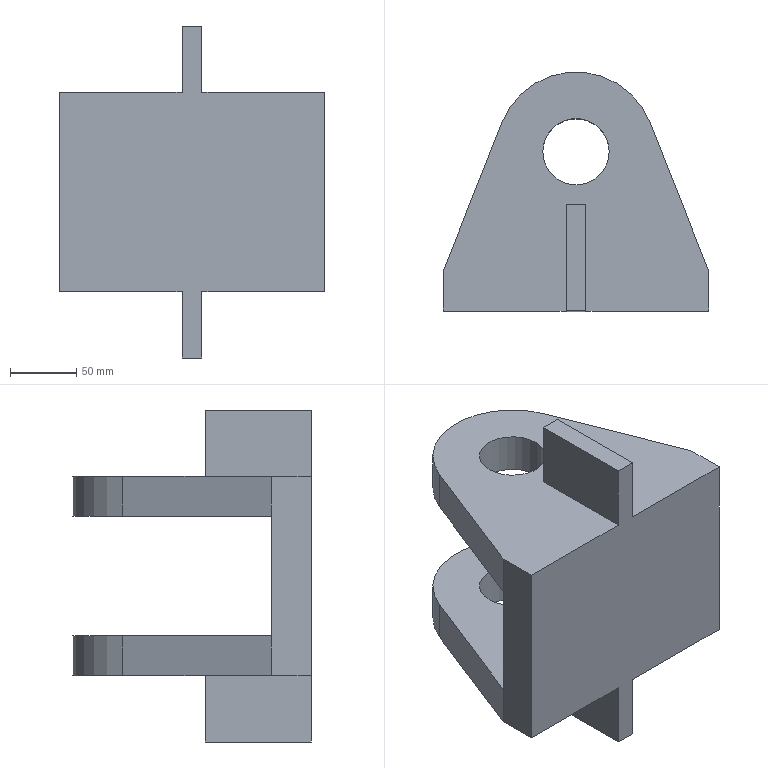Part | SolidWorks | features ICE 2, Extrusion 1, MirrorPattern 1 | 1 solid | 26 faces | box 200 x 180 x 250 mm | volume 2133825 mm3 | plane 20 | cylinder 6 | commonest cylinder face diameters 50 x4 120 x2
STEP:
#1=CARTESIAN_POINT('',(-25.,120.,-45.));
#2=VERTEX_POINT('',#1);
#3=CARTESIAN_POINT('',(25.,120.,-45.));
#4=VERTEX_POINT('',#3);
#5=CARTESIAN_POINT('',(0.,120.,-45.));
#6=DIRECTION('',(0.,0.,1.));
#7=DIRECTION('',(1.,0.,0.));
#8=AXIS2_PLACEMENT_3D('',#5,#6,#7);
#9=CIRCLE('',#8,25.);
#10=EDGE_CURVE('',#2,#4,#9,.T.);
#11=ORIENTED_EDGE('',*,*,#10,.T.);
#12=CARTESIAN_POINT('',(25.,120.,-75.));
#13=VERTEX_POINT('',#12);
#14=CARTESIAN_POINT('',(25.,120.,-45.));
#15=DIRECTION('',(0.,0.,-1.));
#16=VECTOR('',#15,1000.);
#17=LINE('',#14,#16);
#18=EDGE_CURVE('',#4,#13,#17,.T.);
#19=ORIENTED_EDGE('',*,*,#18,.T.);
#20=CARTESIAN_POINT('',(-25.,120.,-75.));
#21=VERTEX_POINT('',#20);
#22=CARTESIAN_POINT('',(0.,120.,-75.));
#23=DIRECTION('',(0.,0.,1.));
#24=DIRECTION('',(1.,0.,0.));
#25=AXIS2_PLACEMENT_3D('',#22,#23,#24);
#26=CIRCLE('',#25,25.);
#27=EDGE_CURVE('',#21,#13,#26,.T.);
#28=ORIENTED_EDGE('',*,*,#27,.F.);
#29=CARTESIAN_POINT('',(-25.,120.,-45.));
#30=DIRECTION('',(0.,0.,-1.));
#31=VECTOR('',#30,1000.);
#32=LINE('',#29,#31);
#33=EDGE_CURVE('',#2,#21,#32,.T.);
#34=ORIENTED_EDGE('',*,*,#33,.F.);
#35=EDGE_LOOP('',(#11,#19,#28,#34));
#36=FACE_OUTER_BOUND('',#35,.T.);
#37=CARTESIAN_POINT('',(0.,120.,-45.));
#38=DIRECTION('',(0.,0.,-1.));
#39=DIRECTION('',(-1.,0.,0.));
#40=AXIS2_PLACEMENT_3D('',#37,#38,#39);
#41=CYLINDRICAL_SURFACE('',#40,25.);
#42=ADVANCED_FACE('',(#36),#41,.F.);
#43=CARTESIAN_POINT('',(-25.,120.,45.));
#44=VERTEX_POINT('',#43);
#45=CARTESIAN_POINT('',(25.,120.,45.));
#46=VERTEX_POINT('',#45);
#47=CARTESIAN_POINT('',(0.,120.,45.));
#48=DIRECTION('',(0.,0.,1.));
#49=DIRECTION('',(1.,0.,0.));
#50=AXIS2_PLACEMENT_3D('',#47,#48,#49);
#51=CIRCLE('',#50,25.);
#52=EDGE_CURVE('',#44,#46,#51,.T.);
#53=ORIENTED_EDGE('',*,*,#52,.F.);
#54=CARTESIAN_POINT('',(-25.,120.,75.));
#55=VERTEX_POINT('',#54);
#56=CARTESIAN_POINT('',(-25.,120.,45.));
#57=DIRECTION('',(0.,0.,1.));
#58=VECTOR('',#57,1000.);
#59=LINE('',#56,#58);
#60=EDGE_CURVE('',#44,#55,#59,.T.);
#61=ORIENTED_EDGE('',*,*,#60,.T.);
#62=CARTESIAN_POINT('',(25.,120.,75.));
#63=VERTEX_POINT('',#62);
#64=CARTESIAN_POINT('',(0.,120.,75.));
#65=DIRECTION('',(0.,0.,1.));
#66=DIRECTION('',(1.,0.,0.));
#67=AXIS2_PLACEMENT_3D('',#64,#65,#66);
#68=CIRCLE('',#67,25.);
#69=EDGE_CURVE('',#55,#63,#68,.T.);
#70=ORIENTED_EDGE('',*,*,#69,.T.);
#71=CARTESIAN_POINT('',(25.,120.,45.));
#72=DIRECTION('',(0.,0.,1.));
#73=VECTOR('',#72,1000.);
#74=LINE('',#71,#73);
#75=EDGE_CURVE('',#46,#63,#74,.T.);
#76=ORIENTED_EDGE('',*,*,#75,.F.);
#77=EDGE_LOOP('',(#53,#61,#70,#76));
#78=FACE_OUTER_BOUND('',#77,.T.);
#79=CARTESIAN_POINT('',(0.,120.,45.));
#80=DIRECTION('',(0.,0.,1.));
#81=DIRECTION('',(1.,0.,0.));
#82=AXIS2_PLACEMENT_3D('',#79,#80,#81);
#83=CYLINDRICAL_SURFACE('',#82,25.);
#84=ADVANCED_FACE('',(#78),#83,.F.);
#85=CARTESIAN_POINT('',(-100.,30.,-45.));
#86=VERTEX_POINT('',#85);
#87=CARTESIAN_POINT('',(100.,30.,-45.));
#88=VERTEX_POINT('',#87);
#89=CARTESIAN_POINT('',(-100.,30.,-45.));
#90=DIRECTION('',(1.,0.,0.));
#91=VECTOR('',#90,1000.);
#92=LINE('',#89,#91);
#93=EDGE_CURVE('',#86,#88,#92,.T.);
#94=ORIENTED_EDGE('',*,*,#93,.F.);
#95=CARTESIAN_POINT('',(-100.,30.,45.));
#96=VERTEX_POINT('',#95);
#97=CARTESIAN_POINT('',(-100.,30.,75.));
#98=DIRECTION('',(0.,0.,1.));
#99=VECTOR('',#98,1000.);
#100=LINE('',#97,#99);
#101=EDGE_CURVE('',#86,#96,#100,.T.);
#102=ORIENTED_EDGE('',*,*,#101,.T.);
#103=CARTESIAN_POINT('',(100.,30.,45.));
#104=VERTEX_POINT('',#103);
#105=CARTESIAN_POINT('',(-100.,30.,45.));
#106=DIRECTION('',(1.,0.,0.));
#107=VECTOR('',#106,1000.);
#108=LINE('',#105,#107);
#109=EDGE_CURVE('',#96,#104,#108,.T.);
#110=ORIENTED_EDGE('',*,*,#109,.T.);
#111=CARTESIAN_POINT('',(100.,30.,75.));
#112=DIRECTION('',(0.,0.,-1.));
#113=VECTOR('',#112,1000.);
#114=LINE('',#111,#113);
#115=EDGE_CURVE('',#104,#88,#114,.T.);
#116=ORIENTED_EDGE('',*,*,#115,.T.);
#117=EDGE_LOOP('',(#94,#102,#110,#116));
#118=FACE_OUTER_BOUND('',#117,.T.);
#119=CARTESIAN_POINT('',(0.,30.,0.));
#120=DIRECTION('',(0.,-1.,0.));
#121=DIRECTION('',(0.,0.,-1.));
#122=AXIS2_PLACEMENT_3D('',#119,#120,#121);
#123=PLANE('',#122);
#124=ADVANCED_FACE('',(#118),#123,.F.);
#125=CARTESIAN_POINT('',(0.,120.,75.));
#126=DIRECTION('',(0.,0.,1.));
#127=DIRECTION('',(1.,0.,0.));
#128=AXIS2_PLACEMENT_3D('',#125,#126,#127);
#129=CIRCLE('',#128,25.);
#130=EDGE_CURVE('',#63,#55,#129,.T.);
#131=ORIENTED_EDGE('',*,*,#130,.F.);
#132=ORIENTED_EDGE('',*,*,#69,.F.);
#133=EDGE_LOOP('',(#131,#132));
#134=FACE_BOUND('',#133,.T.);
#135=CARTESIAN_POINT('',(7.5,0.,75.));
#136=VERTEX_POINT('',#135);
#137=CARTESIAN_POINT('',(7.5,80.,75.));
#138=VERTEX_POINT('',#137);
#139=CARTESIAN_POINT('',(7.5,80.,75.));
#140=DIRECTION('',(0.,1.,0.));
#141=VECTOR('',#140,1000.);
#142=LINE('',#139,#141);
#143=EDGE_CURVE('',#136,#138,#142,.T.);
#144=ORIENTED_EDGE('',*,*,#143,.F.);
#145=CARTESIAN_POINT('',(100.,0.,75.));
#146=VERTEX_POINT('',#145);
#147=CARTESIAN_POINT('',(-100.,0.,75.));
#148=DIRECTION('',(1.,0.,0.));
#149=VECTOR('',#148,1000.);
#150=LINE('',#147,#149);
#151=EDGE_CURVE('',#136,#146,#150,.T.);
#152=ORIENTED_EDGE('',*,*,#151,.T.);
#153=CARTESIAN_POINT('',(100.,30.,75.));
#154=VERTEX_POINT('',#153);
#155=CARTESIAN_POINT('',(100.,30.,75.));
#156=DIRECTION('',(0.,-1.,0.));
#157=VECTOR('',#156,1000.);
#158=LINE('',#155,#157);
#159=EDGE_CURVE('',#154,#146,#158,.T.);
#160=ORIENTED_EDGE('',*,*,#159,.F.);
#161=CARTESIAN_POINT('',(55.815,142.016,75.));
#162=VERTEX_POINT('',#161);
#163=CARTESIAN_POINT('',(55.815,142.016,75.));
#164=DIRECTION('',(-0.3669,0.9302,0.));
#165=VECTOR('',#164,1000.);
#166=LINE('',#163,#165);
#167=EDGE_CURVE('',#154,#162,#166,.T.);
#168=ORIENTED_EDGE('',*,*,#167,.T.);
#169=CARTESIAN_POINT('',(-55.815,142.016,75.));
#170=VERTEX_POINT('',#169);
#171=CARTESIAN_POINT('',(0.,120.,75.));
#172=DIRECTION('',(0.,0.,1.));
#173=DIRECTION('',(1.,0.,0.));
#174=AXIS2_PLACEMENT_3D('',#171,#172,#173);
#175=CIRCLE('',#174,60.);
#176=EDGE_CURVE('',#162,#170,#175,.T.);
#177=ORIENTED_EDGE('',*,*,#176,.T.);
#178=CARTESIAN_POINT('',(-100.,30.,75.));
#179=VERTEX_POINT('',#178);
#180=CARTESIAN_POINT('',(-55.815,142.016,75.));
#181=DIRECTION('',(-0.3669,-0.9302,0.));
#182=VECTOR('',#181,1000.);
#183=LINE('',#180,#182);
#184=EDGE_CURVE('',#170,#179,#183,.T.);
#185=ORIENTED_EDGE('',*,*,#184,.T.);
#186=CARTESIAN_POINT('',(-100.,0.,75.));
#187=VERTEX_POINT('',#186);
#188=CARTESIAN_POINT('',(-100.,30.,75.));
#189=DIRECTION('',(0.,-1.,0.));
#190=VECTOR('',#189,1000.);
#191=LINE('',#188,#190);
#192=EDGE_CURVE('',#179,#187,#191,.T.);
#193=ORIENTED_EDGE('',*,*,#192,.T.);
#194=CARTESIAN_POINT('',(-7.5,0.,75.));
#195=VERTEX_POINT('',#194);
#196=CARTESIAN_POINT('',(-100.,0.,75.));
#197=DIRECTION('',(1.,0.,0.));
#198=VECTOR('',#197,1000.);
#199=LINE('',#196,#198);
#200=EDGE_CURVE('',#187,#195,#199,.T.);
#201=ORIENTED_EDGE('',*,*,#200,.T.);
#202=CARTESIAN_POINT('',(-7.5,80.,75.));
#203=VERTEX_POINT('',#202);
#204=CARTESIAN_POINT('',(-7.5,80.,75.));
#205=DIRECTION('',(0.,-1.,0.));
#206=VECTOR('',#205,1000.);
#207=LINE('',#204,#206);
#208=EDGE_CURVE('',#203,#195,#207,.T.);
#209=ORIENTED_EDGE('',*,*,#208,.F.);
#210=CARTESIAN_POINT('',(-7.5,80.,75.));
#211=DIRECTION('',(-1.,0.,0.));
#212=VECTOR('',#211,1000.);
#213=LINE('',#210,#212);
#214=EDGE_CURVE('',#138,#203,#213,.T.);
#215=ORIENTED_EDGE('',*,*,#214,.F.);
#216=EDGE_LOOP('',(#144,#152,#160,#168,#177,#185,#193,#201,#209,#215));
#217=FACE_OUTER_BOUND('',#216,.T.);
#218=CARTESIAN_POINT('',(-100.,30.,75.));
#219=DIRECTION('',(0.,0.,-1.));
#220=DIRECTION('',(-1.,0.,0.));
#221=AXIS2_PLACEMENT_3D('',#218,#219,#220);
#222=PLANE('',#221);
#223=ADVANCED_FACE('',(#134,#217),#222,.F.);
#224=CARTESIAN_POINT('',(100.,0.,-75.));
#225=VERTEX_POINT('',#224);
#226=CARTESIAN_POINT('',(100.,0.,75.));
#227=DIRECTION('',(0.,0.,-1.));
#228=VECTOR('',#227,1000.);
#229=LINE('',#226,#228);
#230=EDGE_CURVE('',#146,#225,#229,.T.);
#231=ORIENTED_EDGE('',*,*,#230,.T.);
#232=CARTESIAN_POINT('',(100.,30.,-75.));
#233=VERTEX_POINT('',#232);
#234=CARTESIAN_POINT('',(100.,30.,-75.));
#235=DIRECTION('',(0.,-1.,0.));
#236=VECTOR('',#235,1000.);
#237=LINE('',#234,#236);
#238=EDGE_CURVE('',#233,#225,#237,.T.);
#239=ORIENTED_EDGE('',*,*,#238,.F.);
#240=CARTESIAN_POINT('',(100.,30.,-45.));
#241=DIRECTION('',(0.,0.,-1.));
#242=VECTOR('',#241,1000.);
#243=LINE('',#240,#242);
#244=EDGE_CURVE('',#88,#233,#243,.T.);
#245=ORIENTED_EDGE('',*,*,#244,.F.);
#246=ORIENTED_EDGE('',*,*,#115,.F.);
#247=CARTESIAN_POINT('',(100.,30.,75.));
#248=DIRECTION('',(0.,0.,-1.));
#249=VECTOR('',#248,1000.);
#250=LINE('',#247,#249);
#251=EDGE_CURVE('',#154,#104,#250,.T.);
#252=ORIENTED_EDGE('',*,*,#251,.F.);
#253=ORIENTED_EDGE('',*,*,#159,.T.);
#254=EDGE_LOOP('',(#231,#239,#245,#246,#252,#253));
#255=FACE_OUTER_BOUND('',#254,.T.);
#256=CARTESIAN_POINT('',(100.,30.,75.));
#257=DIRECTION('',(-1.,0.,0.));
#258=DIRECTION('',(0.,0.,1.));
#259=AXIS2_PLACEMENT_3D('',#256,#257,#258);
#260=PLANE('',#259);
#261=ADVANCED_FACE('',(#255),#260,.F.);
#262=CARTESIAN_POINT('',(7.5,0.,-75.));
#263=VERTEX_POINT('',#262);
#264=CARTESIAN_POINT('',(-100.,0.,-75.));
#265=DIRECTION('',(-1.,0.,0.));
#266=VECTOR('',#265,1000.);
#267=LINE('',#264,#266);
#268=EDGE_CURVE('',#225,#263,#267,.T.);
#269=ORIENTED_EDGE('',*,*,#268,.T.);
#270=CARTESIAN_POINT('',(7.5,80.,-75.));
#271=VERTEX_POINT('',#270);
#272=CARTESIAN_POINT('',(7.5,80.,-75.));
#273=DIRECTION('',(0.,1.,0.));
#274=VECTOR('',#273,1000.);
#275=LINE('',#272,#274);
#276=EDGE_CURVE('',#263,#271,#275,.T.);
#277=ORIENTED_EDGE('',*,*,#276,.T.);
#278=CARTESIAN_POINT('',(-7.5,80.,-75.));
#279=VERTEX_POINT('',#278);
#280=CARTESIAN_POINT('',(-7.5,80.,-75.));
#281=DIRECTION('',(-1.,0.,0.));
#282=VECTOR('',#281,1000.);
#283=LINE('',#280,#282);
#284=EDGE_CURVE('',#271,#279,#283,.T.);
#285=ORIENTED_EDGE('',*,*,#284,.T.);
#286=CARTESIAN_POINT('',(-7.5,0.,-75.));
#287=VERTEX_POINT('',#286);
#288=CARTESIAN_POINT('',(-7.5,80.,-75.));
#289=DIRECTION('',(0.,-1.,0.));
#290=VECTOR('',#289,1000.);
#291=LINE('',#288,#290);
#292=EDGE_CURVE('',#279,#287,#291,.T.);
#293=ORIENTED_EDGE('',*,*,#292,.T.);
#294=CARTESIAN_POINT('',(-100.,0.,-75.));
#295=VERTEX_POINT('',#294);
#296=CARTESIAN_POINT('',(-100.,0.,-75.));
#297=DIRECTION('',(-1.,0.,0.));
#298=VECTOR('',#297,1000.);
#299=LINE('',#296,#298);
#300=EDGE_CURVE('',#287,#295,#299,.T.);
#301=ORIENTED_EDGE('',*,*,#300,.T.);
#302=CARTESIAN_POINT('',(-100.,30.,-75.));
#303=VERTEX_POINT('',#302);
#304=CARTESIAN_POINT('',(-100.,30.,-75.));
#305=DIRECTION('',(0.,-1.,0.));
#306=VECTOR('',#305,1000.);
#307=LINE('',#304,#306);
#308=EDGE_CURVE('',#303,#295,#307,.T.);
#309=ORIENTED_EDGE('',*,*,#308,.F.);
#310=CARTESIAN_POINT('',(-55.815,142.016,-75.));
#311=VERTEX_POINT('',#310);
#312=CARTESIAN_POINT('',(-55.815,142.016,-75.));
#313=DIRECTION('',(-0.3669,-0.9302,0.));
#314=VECTOR('',#313,1000.);
#315=LINE('',#312,#314);
#316=EDGE_CURVE('',#311,#303,#315,.T.);
#317=ORIENTED_EDGE('',*,*,#316,.F.);
#318=CARTESIAN_POINT('',(55.815,142.016,-75.));
#319=VERTEX_POINT('',#318);
#320=CARTESIAN_POINT('',(0.,120.,-75.));
#321=DIRECTION('',(0.,0.,1.));
#322=DIRECTION('',(1.,0.,0.));
#323=AXIS2_PLACEMENT_3D('',#320,#321,#322);
#324=CIRCLE('',#323,60.);
#325=EDGE_CURVE('',#319,#311,#324,.T.);
#326=ORIENTED_EDGE('',*,*,#325,.F.);
#327=CARTESIAN_POINT('',(55.815,142.016,-75.));
#328=DIRECTION('',(-0.3669,0.9302,0.));
#329=VECTOR('',#328,1000.);
#330=LINE('',#327,#329);
#331=EDGE_CURVE('',#233,#319,#330,.T.);
#332=ORIENTED_EDGE('',*,*,#331,.F.);
#333=ORIENTED_EDGE('',*,*,#238,.T.);
#334=EDGE_LOOP('',(#269,#277,#285,#293,#301,#309,#317,#326,#332,#333));
#335=FACE_OUTER_BOUND('',#334,.T.);
#336=ORIENTED_EDGE('',*,*,#27,.T.);
#337=CARTESIAN_POINT('',(0.,120.,-75.));
#338=DIRECTION('',(0.,0.,1.));
#339=DIRECTION('',(1.,0.,0.));
#340=AXIS2_PLACEMENT_3D('',#337,#338,#339);
#341=CIRCLE('',#340,25.);
#342=EDGE_CURVE('',#13,#21,#341,.T.);
#343=ORIENTED_EDGE('',*,*,#342,.T.);
#344=EDGE_LOOP('',(#336,#343));
#345=FACE_BOUND('',#344,.T.);
#346=CARTESIAN_POINT('',(-100.,30.,-75.));
#347=DIRECTION('',(0.,0.,1.));
#348=DIRECTION('',(1.,0.,0.));
#349=AXIS2_PLACEMENT_3D('',#346,#347,#348);
#350=PLANE('',#349);
#351=ADVANCED_FACE('',(#335,#345),#350,.F.);
#352=CARTESIAN_POINT('',(-100.,0.,75.));
#353=DIRECTION('',(0.,0.,1.));
#354=VECTOR('',#353,1000.);
#355=LINE('',#352,#354);
#356=EDGE_CURVE('',#295,#187,#355,.T.);
#357=ORIENTED_EDGE('',*,*,#356,.T.);
#358=ORIENTED_EDGE('',*,*,#192,.F.);
#359=CARTESIAN_POINT('',(-100.,30.,45.));
#360=DIRECTION('',(0.,0.,1.));
#361=VECTOR('',#360,1000.);
#362=LINE('',#359,#361);
#363=EDGE_CURVE('',#96,#179,#362,.T.);
#364=ORIENTED_EDGE('',*,*,#363,.F.);
#365=ORIENTED_EDGE('',*,*,#101,.F.);
#366=CARTESIAN_POINT('',(-100.,30.,75.));
#367=DIRECTION('',(0.,0.,1.));
#368=VECTOR('',#367,1000.);
#369=LINE('',#366,#368);
#370=EDGE_CURVE('',#303,#86,#369,.T.);
#371=ORIENTED_EDGE('',*,*,#370,.F.);
#372=ORIENTED_EDGE('',*,*,#308,.T.);
#373=EDGE_LOOP('',(#357,#358,#364,#365,#371,#372));
#374=FACE_OUTER_BOUND('',#373,.T.);
#375=CARTESIAN_POINT('',(-100.,30.,75.));
#376=DIRECTION('',(1.,0.,0.));
#377=DIRECTION('',(0.,0.,-1.));
#378=AXIS2_PLACEMENT_3D('',#375,#376,#377);
#379=PLANE('',#378);
#380=ADVANCED_FACE('',(#374),#379,.F.);
#381=ORIENTED_EDGE('',*,*,#230,.F.);
#382=ORIENTED_EDGE('',*,*,#151,.F.);
#383=CARTESIAN_POINT('',(7.5,0.,125.));
#384=VERTEX_POINT('',#383);
#385=CARTESIAN_POINT('',(7.5,0.,125.));
#386=DIRECTION('',(0.,0.,-1.));
#387=VECTOR('',#386,1000.);
#388=LINE('',#385,#387);
#389=EDGE_CURVE('',#384,#136,#388,.T.);
#390=ORIENTED_EDGE('',*,*,#389,.F.);
#391=CARTESIAN_POINT('',(-7.5,0.,125.));
#392=VERTEX_POINT('',#391);
#393=CARTESIAN_POINT('',(-7.5,0.,125.));
#394=DIRECTION('',(1.,0.,0.));
#395=VECTOR('',#394,1000.);
#396=LINE('',#393,#395);
#397=EDGE_CURVE('',#392,#384,#396,.T.);
#398=ORIENTED_EDGE('',*,*,#397,.F.);
#399=CARTESIAN_POINT('',(-7.5,0.,125.));
#400=DIRECTION('',(0.,0.,-1.));
#401=VECTOR('',#400,1000.);
#402=LINE('',#399,#401);
#403=EDGE_CURVE('',#392,#195,#402,.T.);
#404=ORIENTED_EDGE('',*,*,#403,.T.);
#405=ORIENTED_EDGE('',*,*,#200,.F.);
#406=ORIENTED_EDGE('',*,*,#356,.F.);
#407=ORIENTED_EDGE('',*,*,#300,.F.);
#408=CARTESIAN_POINT('',(-7.5,0.,-125.));
#409=VERTEX_POINT('',#408);
#410=CARTESIAN_POINT('',(-7.5,0.,-125.));
#411=DIRECTION('',(0.,0.,1.));
#412=VECTOR('',#411,1000.);
#413=LINE('',#410,#412);
#414=EDGE_CURVE('',#409,#287,#413,.T.);
#415=ORIENTED_EDGE('',*,*,#414,.F.);
#416=CARTESIAN_POINT('',(7.5,0.,-125.));
#417=VERTEX_POINT('',#416);
#418=CARTESIAN_POINT('',(-7.5,0.,-125.));
#419=DIRECTION('',(1.,0.,0.));
#420=VECTOR('',#419,1000.);
#421=LINE('',#418,#420);
#422=EDGE_CURVE('',#409,#417,#421,.T.);
#423=ORIENTED_EDGE('',*,*,#422,.T.);
#424=CARTESIAN_POINT('',(7.5,0.,-125.));
#425=DIRECTION('',(0.,0.,1.));
#426=VECTOR('',#425,1000.);
#427=LINE('',#424,#426);
#428=EDGE_CURVE('',#417,#263,#427,.T.);
#429=ORIENTED_EDGE('',*,*,#428,.T.);
#430=ORIENTED_EDGE('',*,*,#268,.F.);
#431=EDGE_LOOP('',(#381,#382,#390,#398,#404,#405,#406,#407,#415,#423,#429,#430));
#432=FACE_OUTER_BOUND('',#431,.T.);
#433=CARTESIAN_POINT('',(0.,0.,0.));
#434=DIRECTION('',(0.,-1.,0.));
#435=DIRECTION('',(0.,0.,-1.));
#436=AXIS2_PLACEMENT_3D('',#433,#434,#435);
#437=PLANE('',#436);
#438=ADVANCED_FACE('',(#432),#437,.T.);
#439=ORIENTED_EDGE('',*,*,#176,.F.);
#440=CARTESIAN_POINT('',(55.815,142.016,45.));
#441=VERTEX_POINT('',#440);
#442=CARTESIAN_POINT('',(55.815,142.016,45.));
#443=DIRECTION('',(0.,0.,1.));
#444=VECTOR('',#443,1000.);
#445=LINE('',#442,#444);
#446=EDGE_CURVE('',#441,#162,#445,.T.);
#447=ORIENTED_EDGE('',*,*,#446,.F.);
#448=CARTESIAN_POINT('',(-55.815,142.016,45.));
#449=VERTEX_POINT('',#448);
#450=CARTESIAN_POINT('',(0.,120.,45.));
#451=DIRECTION('',(0.,0.,1.));
#452=DIRECTION('',(1.,0.,0.));
#453=AXIS2_PLACEMENT_3D('',#450,#451,#452);
#454=CIRCLE('',#453,60.);
#455=EDGE_CURVE('',#441,#449,#454,.T.);
#456=ORIENTED_EDGE('',*,*,#455,.T.);
#457=CARTESIAN_POINT('',(-55.815,142.016,45.));
#458=DIRECTION('',(0.,0.,1.));
#459=VECTOR('',#458,1000.);
#460=LINE('',#457,#459);
#461=EDGE_CURVE('',#449,#170,#460,.T.);
#462=ORIENTED_EDGE('',*,*,#461,.T.);
#463=EDGE_LOOP('',(#439,#447,#456,#462));
#464=FACE_OUTER_BOUND('',#463,.T.);
#465=CARTESIAN_POINT('',(0.,120.,45.));
#466=DIRECTION('',(0.,0.,1.));
#467=DIRECTION('',(1.,0.,0.));
#468=AXIS2_PLACEMENT_3D('',#465,#466,#467);
#469=CYLINDRICAL_SURFACE('',#468,60.);
#470=ADVANCED_FACE('',(#464),#469,.T.);
#471=ORIENTED_EDGE('',*,*,#167,.F.);
#472=ORIENTED_EDGE('',*,*,#251,.T.);
#473=CARTESIAN_POINT('',(55.815,142.016,45.));
#474=DIRECTION('',(-0.3669,0.9302,0.));
#475=VECTOR('',#474,1000.);
#476=LINE('',#473,#475);
#477=EDGE_CURVE('',#104,#441,#476,.T.);
#478=ORIENTED_EDGE('',*,*,#477,.T.);
#479=ORIENTED_EDGE('',*,*,#446,.T.);
#480=EDGE_LOOP('',(#471,#472,#478,#479));
#481=FACE_OUTER_BOUND('',#480,.T.);
#482=CARTESIAN_POINT('',(55.815,142.016,45.));
#483=DIRECTION('',(0.9302,0.3669,0.));
#484=DIRECTION('',(-0.3669,0.9302,0.));
#485=AXIS2_PLACEMENT_3D('',#482,#483,#484);
#486=PLANE('',#485);
#487=ADVANCED_FACE('',(#481),#486,.T.);
#488=ORIENTED_EDGE('',*,*,#184,.F.);
#489=ORIENTED_EDGE('',*,*,#461,.F.);
#490=CARTESIAN_POINT('',(-55.815,142.016,45.));
#491=DIRECTION('',(-0.3669,-0.9302,0.));
#492=VECTOR('',#491,1000.);
#493=LINE('',#490,#492);
#494=EDGE_CURVE('',#449,#96,#493,.T.);
#495=ORIENTED_EDGE('',*,*,#494,.T.);
#496=ORIENTED_EDGE('',*,*,#363,.T.);
#497=EDGE_LOOP('',(#488,#489,#495,#496));
#498=FACE_OUTER_BOUND('',#497,.T.);
#499=CARTESIAN_POINT('',(-55.815,142.016,45.));
#500=DIRECTION('',(-0.9302,0.3669,0.));
#501=DIRECTION('',(-0.3669,-0.9302,0.));
#502=AXIS2_PLACEMENT_3D('',#499,#500,#501);
#503=PLANE('',#502);
#504=ADVANCED_FACE('',(#498),#503,.T.);
#505=CARTESIAN_POINT('',(0.,120.,45.));
#506=DIRECTION('',(0.,0.,1.));
#507=DIRECTION('',(1.,0.,0.));
#508=AXIS2_PLACEMENT_3D('',#505,#506,#507);
#509=CIRCLE('',#508,25.);
#510=EDGE_CURVE('',#46,#44,#509,.T.);
#511=ORIENTED_EDGE('',*,*,#510,.T.);
#512=ORIENTED_EDGE('',*,*,#52,.T.);
#513=EDGE_LOOP('',(#511,#512));
#514=FACE_BOUND('',#513,.T.);
#515=ORIENTED_EDGE('',*,*,#455,.F.);
#516=ORIENTED_EDGE('',*,*,#477,.F.);
#517=ORIENTED_EDGE('',*,*,#109,.F.);
#518=ORIENTED_EDGE('',*,*,#494,.F.);
#519=EDGE_LOOP('',(#515,#516,#517,#518));
#520=FACE_OUTER_BOUND('',#519,.T.);
#521=CARTESIAN_POINT('',(0.,120.,45.));
#522=DIRECTION('',(0.,0.,1.));
#523=DIRECTION('',(1.,0.,0.));
#524=AXIS2_PLACEMENT_3D('',#521,#522,#523);
#525=PLANE('',#524);
#526=ADVANCED_FACE('',(#514,#520),#525,.F.);
#527=ORIENTED_EDGE('',*,*,#60,.F.);
#528=ORIENTED_EDGE('',*,*,#510,.F.);
#529=ORIENTED_EDGE('',*,*,#75,.T.);
#530=ORIENTED_EDGE('',*,*,#130,.T.);
#531=EDGE_LOOP('',(#527,#528,#529,#530));
#532=FACE_OUTER_BOUND('',#531,.T.);
#533=CARTESIAN_POINT('',(0.,120.,45.));
#534=DIRECTION('',(0.,0.,1.));
#535=DIRECTION('',(1.,0.,0.));
#536=AXIS2_PLACEMENT_3D('',#533,#534,#535);
#537=CYLINDRICAL_SURFACE('',#536,25.);
#538=ADVANCED_FACE('',(#532),#537,.F.);
#539=ORIENTED_EDGE('',*,*,#143,.T.);
#540=CARTESIAN_POINT('',(7.5,80.,125.));
#541=VERTEX_POINT('',#540);
#542=CARTESIAN_POINT('',(7.5,80.,125.));
#543=DIRECTION('',(0.,0.,-1.));
#544=VECTOR('',#543,1000.);
#545=LINE('',#542,#544);
#546=EDGE_CURVE('',#541,#138,#545,.T.);
#547=ORIENTED_EDGE('',*,*,#546,.F.);
#548=CARTESIAN_POINT('',(7.5,80.,125.));
#549=DIRECTION('',(0.,1.,0.));
#550=VECTOR('',#549,1000.);
#551=LINE('',#548,#550);
#552=EDGE_CURVE('',#384,#541,#551,.T.);
#553=ORIENTED_EDGE('',*,*,#552,.F.);
#554=ORIENTED_EDGE('',*,*,#389,.T.);
#555=EDGE_LOOP('',(#539,#547,#553,#554));
#556=FACE_OUTER_BOUND('',#555,.T.);
#557=CARTESIAN_POINT('',(7.5,80.,125.));
#558=DIRECTION('',(-1.,0.,0.));
#559=DIRECTION('',(0.,-1.,0.));
#560=AXIS2_PLACEMENT_3D('',#557,#558,#559);
#561=PLANE('',#560);
#562=ADVANCED_FACE('',(#556),#561,.F.);
#563=ORIENTED_EDGE('',*,*,#214,.T.);
#564=CARTESIAN_POINT('',(-7.5,80.,125.));
#565=VERTEX_POINT('',#564);
#566=CARTESIAN_POINT('',(-7.5,80.,125.));
#567=DIRECTION('',(0.,0.,-1.));
#568=VECTOR('',#567,1000.);
#569=LINE('',#566,#568);
#570=EDGE_CURVE('',#565,#203,#569,.T.);
#571=ORIENTED_EDGE('',*,*,#570,.F.);
#572=CARTESIAN_POINT('',(-7.5,80.,125.));
#573=DIRECTION('',(-1.,0.,0.));
#574=VECTOR('',#573,1000.);
#575=LINE('',#572,#574);
#576=EDGE_CURVE('',#541,#565,#575,.T.);
#577=ORIENTED_EDGE('',*,*,#576,.F.);
#578=ORIENTED_EDGE('',*,*,#546,.T.);
#579=EDGE_LOOP('',(#563,#571,#577,#578));
#580=FACE_OUTER_BOUND('',#579,.T.);
#581=CARTESIAN_POINT('',(-7.5,80.,125.));
#582=DIRECTION('',(0.,-1.,0.));
#583=DIRECTION('',(0.,0.,-1.));
#584=AXIS2_PLACEMENT_3D('',#581,#582,#583);
#585=PLANE('',#584);
#586=ADVANCED_FACE('',(#580),#585,.F.);
#587=ORIENTED_EDGE('',*,*,#208,.T.);
#588=ORIENTED_EDGE('',*,*,#403,.F.);
#589=CARTESIAN_POINT('',(-7.5,80.,125.));
#590=DIRECTION('',(0.,-1.,0.));
#591=VECTOR('',#590,1000.);
#592=LINE('',#589,#591);
#593=EDGE_CURVE('',#565,#392,#592,.T.);
#594=ORIENTED_EDGE('',*,*,#593,.F.);
#595=ORIENTED_EDGE('',*,*,#570,.T.);
#596=EDGE_LOOP('',(#587,#588,#594,#595));
#597=FACE_OUTER_BOUND('',#596,.T.);
#598=CARTESIAN_POINT('',(-7.5,80.,125.));
#599=DIRECTION('',(1.,0.,0.));
#600=DIRECTION('',(0.,1.,0.));
#601=AXIS2_PLACEMENT_3D('',#598,#599,#600);
#602=PLANE('',#601);
#603=ADVANCED_FACE('',(#597),#602,.F.);
#604=ORIENTED_EDGE('',*,*,#552,.T.);
#605=ORIENTED_EDGE('',*,*,#576,.T.);
#606=ORIENTED_EDGE('',*,*,#593,.T.);
#607=ORIENTED_EDGE('',*,*,#397,.T.);
#608=EDGE_LOOP('',(#604,#605,#606,#607));
#609=FACE_OUTER_BOUND('',#608,.T.);
#610=CARTESIAN_POINT('',(0.,0.,125.));
#611=DIRECTION('',(0.,0.,1.));
#612=DIRECTION('',(1.,0.,0.));
#613=AXIS2_PLACEMENT_3D('',#610,#611,#612);
#614=PLANE('',#613);
#615=ADVANCED_FACE('',(#609),#614,.T.);
#616=CARTESIAN_POINT('',(55.815,142.016,-45.));
#617=VERTEX_POINT('',#616);
#618=CARTESIAN_POINT('',(-55.815,142.016,-45.));
#619=VERTEX_POINT('',#618);
#620=CARTESIAN_POINT('',(0.,120.,-45.));
#621=DIRECTION('',(0.,0.,1.));
#622=DIRECTION('',(1.,0.,0.));
#623=AXIS2_PLACEMENT_3D('',#620,#621,#622);
#624=CIRCLE('',#623,60.);
#625=EDGE_CURVE('',#617,#619,#624,.T.);
#626=ORIENTED_EDGE('',*,*,#625,.T.);
#627=CARTESIAN_POINT('',(-55.815,142.016,-45.));
#628=DIRECTION('',(-0.3669,-0.9302,0.));
#629=VECTOR('',#628,1000.);
#630=LINE('',#627,#629);
#631=EDGE_CURVE('',#619,#86,#630,.T.);
#632=ORIENTED_EDGE('',*,*,#631,.T.);
#633=ORIENTED_EDGE('',*,*,#93,.T.);
#634=CARTESIAN_POINT('',(55.815,142.016,-45.));
#635=DIRECTION('',(-0.3669,0.9302,0.));
#636=VECTOR('',#635,1000.);
#637=LINE('',#634,#636);
#638=EDGE_CURVE('',#88,#617,#637,.T.);
#639=ORIENTED_EDGE('',*,*,#638,.T.);
#640=EDGE_LOOP('',(#626,#632,#633,#639));
#641=FACE_OUTER_BOUND('',#640,.T.);
#642=ORIENTED_EDGE('',*,*,#10,.F.);
#643=CARTESIAN_POINT('',(0.,120.,-45.));
#644=DIRECTION('',(0.,0.,1.));
#645=DIRECTION('',(1.,0.,0.));
#646=AXIS2_PLACEMENT_3D('',#643,#644,#645);
#647=CIRCLE('',#646,25.);
#648=EDGE_CURVE('',#4,#2,#647,.T.);
#649=ORIENTED_EDGE('',*,*,#648,.F.);
#650=EDGE_LOOP('',(#642,#649));
#651=FACE_BOUND('',#650,.T.);
#652=CARTESIAN_POINT('',(0.,120.,-45.));
#653=DIRECTION('',(0.,0.,-1.));
#654=DIRECTION('',(1.,0.,0.));
#655=AXIS2_PLACEMENT_3D('',#652,#653,#654);
#656=PLANE('',#655);
#657=ADVANCED_FACE('',(#641,#651),#656,.F.);
#658=ORIENTED_EDGE('',*,*,#325,.T.);
#659=CARTESIAN_POINT('',(-55.815,142.016,-45.));
#660=DIRECTION('',(0.,0.,-1.));
#661=VECTOR('',#660,1000.);
#662=LINE('',#659,#661);
#663=EDGE_CURVE('',#619,#311,#662,.T.);
#664=ORIENTED_EDGE('',*,*,#663,.F.);
#665=ORIENTED_EDGE('',*,*,#625,.F.);
#666=CARTESIAN_POINT('',(55.815,142.016,-45.));
#667=DIRECTION('',(0.,0.,-1.));
#668=VECTOR('',#667,1000.);
#669=LINE('',#666,#668);
#670=EDGE_CURVE('',#617,#319,#669,.T.);
#671=ORIENTED_EDGE('',*,*,#670,.T.);
#672=EDGE_LOOP('',(#658,#664,#665,#671));
#673=FACE_OUTER_BOUND('',#672,.T.);
#674=CARTESIAN_POINT('',(0.,120.,-45.));
#675=DIRECTION('',(0.,0.,-1.));
#676=DIRECTION('',(-1.,0.,0.));
#677=AXIS2_PLACEMENT_3D('',#674,#675,#676);
#678=CYLINDRICAL_SURFACE('',#677,60.);
#679=ADVANCED_FACE('',(#673),#678,.T.);
#680=ORIENTED_EDGE('',*,*,#316,.T.);
#681=ORIENTED_EDGE('',*,*,#370,.T.);
#682=ORIENTED_EDGE('',*,*,#631,.F.);
#683=ORIENTED_EDGE('',*,*,#663,.T.);
#684=EDGE_LOOP('',(#680,#681,#682,#683));
#685=FACE_OUTER_BOUND('',#684,.T.);
#686=CARTESIAN_POINT('',(-55.815,142.016,-45.));
#687=DIRECTION('',(0.9302,-0.3669,0.));
#688=DIRECTION('',(0.3669,0.9302,0.));
#689=AXIS2_PLACEMENT_3D('',#686,#687,#688);
#690=PLANE('',#689);
#691=ADVANCED_FACE('',(#685),#690,.F.);
#692=ORIENTED_EDGE('',*,*,#331,.T.);
#693=ORIENTED_EDGE('',*,*,#670,.F.);
#694=ORIENTED_EDGE('',*,*,#638,.F.);
#695=ORIENTED_EDGE('',*,*,#244,.T.);
#696=EDGE_LOOP('',(#692,#693,#694,#695));
#697=FACE_OUTER_BOUND('',#696,.T.);
#698=CARTESIAN_POINT('',(55.815,142.016,-45.));
#699=DIRECTION('',(-0.9302,-0.3669,0.));
#700=DIRECTION('',(0.3669,-0.9302,0.));
#701=AXIS2_PLACEMENT_3D('',#698,#699,#700);
#702=PLANE('',#701);
#703=ADVANCED_FACE('',(#697),#702,.F.);
#704=ORIENTED_EDGE('',*,*,#18,.F.);
#705=ORIENTED_EDGE('',*,*,#648,.T.);
#706=ORIENTED_EDGE('',*,*,#33,.T.);
#707=ORIENTED_EDGE('',*,*,#342,.F.);
#708=EDGE_LOOP('',(#704,#705,#706,#707));
#709=FACE_OUTER_BOUND('',#708,.T.);
#710=CARTESIAN_POINT('',(0.,120.,-45.));
#711=DIRECTION('',(0.,0.,-1.));
#712=DIRECTION('',(-1.,0.,0.));
#713=AXIS2_PLACEMENT_3D('',#710,#711,#712);
#714=CYLINDRICAL_SURFACE('',#713,25.);
#715=ADVANCED_FACE('',(#709),#714,.F.);
#716=ORIENTED_EDGE('',*,*,#276,.F.);
#717=ORIENTED_EDGE('',*,*,#428,.F.);
#718=CARTESIAN_POINT('',(7.5,80.,-125.));
#719=VERTEX_POINT('',#718);
#720=CARTESIAN_POINT('',(7.5,80.,-125.));
#721=DIRECTION('',(0.,1.,0.));
#722=VECTOR('',#721,1000.);
#723=LINE('',#720,#722);
#724=EDGE_CURVE('',#417,#719,#723,.T.);
#725=ORIENTED_EDGE('',*,*,#724,.T.);
#726=CARTESIAN_POINT('',(7.5,80.,-125.));
#727=DIRECTION('',(0.,0.,1.));
#728=VECTOR('',#727,1000.);
#729=LINE('',#726,#728);
#730=EDGE_CURVE('',#719,#271,#729,.T.);
#731=ORIENTED_EDGE('',*,*,#730,.T.);
#732=EDGE_LOOP('',(#716,#717,#725,#731));
#733=FACE_OUTER_BOUND('',#732,.T.);
#734=CARTESIAN_POINT('',(7.5,80.,-125.));
#735=DIRECTION('',(1.,0.,0.));
#736=DIRECTION('',(0.,1.,0.));
#737=AXIS2_PLACEMENT_3D('',#734,#735,#736);
#738=PLANE('',#737);
#739=ADVANCED_FACE('',(#733),#738,.T.);
#740=ORIENTED_EDGE('',*,*,#292,.F.);
#741=CARTESIAN_POINT('',(-7.5,80.,-125.));
#742=VERTEX_POINT('',#741);
#743=CARTESIAN_POINT('',(-7.5,80.,-125.));
#744=DIRECTION('',(0.,0.,1.));
#745=VECTOR('',#744,1000.);
#746=LINE('',#743,#745);
#747=EDGE_CURVE('',#742,#279,#746,.T.);
#748=ORIENTED_EDGE('',*,*,#747,.F.);
#749=CARTESIAN_POINT('',(-7.5,80.,-125.));
#750=DIRECTION('',(0.,-1.,0.));
#751=VECTOR('',#750,1000.);
#752=LINE('',#749,#751);
#753=EDGE_CURVE('',#742,#409,#752,.T.);
#754=ORIENTED_EDGE('',*,*,#753,.T.);
#755=ORIENTED_EDGE('',*,*,#414,.T.);
#756=EDGE_LOOP('',(#740,#748,#754,#755));
#757=FACE_OUTER_BOUND('',#756,.T.);
#758=CARTESIAN_POINT('',(-7.5,80.,-125.));
#759=DIRECTION('',(-1.,0.,0.));
#760=DIRECTION('',(0.,-1.,0.));
#761=AXIS2_PLACEMENT_3D('',#758,#759,#760);
#762=PLANE('',#761);
#763=ADVANCED_FACE('',(#757),#762,.T.);
#764=ORIENTED_EDGE('',*,*,#284,.F.);
#765=ORIENTED_EDGE('',*,*,#730,.F.);
#766=CARTESIAN_POINT('',(-7.5,80.,-125.));
#767=DIRECTION('',(-1.,0.,0.));
#768=VECTOR('',#767,1000.);
#769=LINE('',#766,#768);
#770=EDGE_CURVE('',#719,#742,#769,.T.);
#771=ORIENTED_EDGE('',*,*,#770,.T.);
#772=ORIENTED_EDGE('',*,*,#747,.T.);
#773=EDGE_LOOP('',(#764,#765,#771,#772));
#774=FACE_OUTER_BOUND('',#773,.T.);
#775=CARTESIAN_POINT('',(-7.5,80.,-125.));
#776=DIRECTION('',(0.,1.,0.));
#777=DIRECTION('',(0.,0.,1.));
#778=AXIS2_PLACEMENT_3D('',#775,#776,#777);
#779=PLANE('',#778);
#780=ADVANCED_FACE('',(#774),#779,.T.);
#781=ORIENTED_EDGE('',*,*,#724,.F.);
#782=ORIENTED_EDGE('',*,*,#422,.F.);
#783=ORIENTED_EDGE('',*,*,#753,.F.);
#784=ORIENTED_EDGE('',*,*,#770,.F.);
#785=EDGE_LOOP('',(#781,#782,#783,#784));
#786=FACE_OUTER_BOUND('',#785,.T.);
#787=CARTESIAN_POINT('',(0.,0.,-125.));
#788=DIRECTION('',(0.,0.,-1.));
#789=DIRECTION('',(1.,0.,0.));
#790=AXIS2_PLACEMENT_3D('',#787,#788,#789);
#791=PLANE('',#790);
#792=ADVANCED_FACE('',(#786),#791,.T.);
#793=CLOSED_SHELL('',(#42,#84,#124,#223,#261,#351,#380,#438,#470,#487,#504,#526,#538,#562,#586,#603,#615,#657,#679,#691,#703,#715,#739,#763,#780,#792));
#794=MANIFOLD_SOLID_BREP('',#793);
#795=CARTESIAN_POINT('',(0.,0.,0.));
#796=DIRECTION('',(0.,0.,1.));
#797=DIRECTION('',(1.,0.,0.));
#798=AXIS2_PLACEMENT_3D('',#795,#796,#797);
#799=(LENGTH_UNIT()NAMED_UNIT(*)SI_UNIT(.MILLI.,.METRE.));
#800=UNCERTAINTY_MEASURE_WITH_UNIT(LENGTH_MEASURE(0.00001),#799,'','');
#801=(NAMED_UNIT(*)PLANE_ANGLE_UNIT()SI_UNIT($,.RADIAN.));
#802=(NAMED_UNIT(*)SI_UNIT($,.STERADIAN.)SOLID_ANGLE_UNIT());
#803=(GEOMETRIC_REPRESENTATION_CONTEXT(3)GLOBAL_UNCERTAINTY_ASSIGNED_CONTEXT((#800))GLOBAL_UNIT_ASSIGNED_CONTEXT((#799,#801,#802))REPRESENTATION_CONTEXT('',''));
#804=ADVANCED_BREP_SHAPE_REPRESENTATION('',(#794,#798),#803);